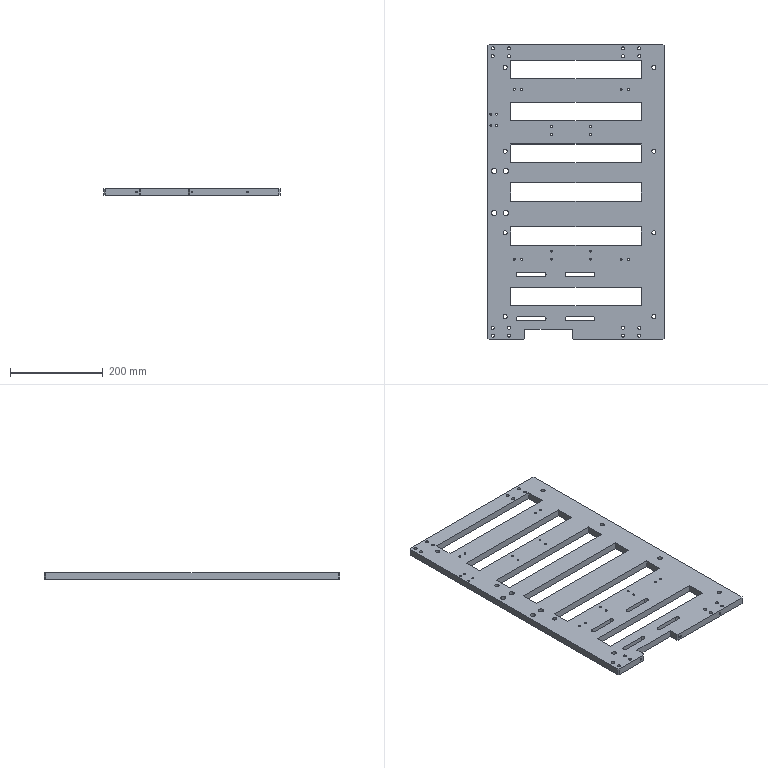Part | STEP file | 1 solid | 196 faces | box 380 x 636 x 15 mm | volume 2517055 mm3 | cylinder 128 | plane 54 | cone 14 | commonest cylinder face diameters 4.2 x52 6.8 x32 9 x28 11 x8 17 x8